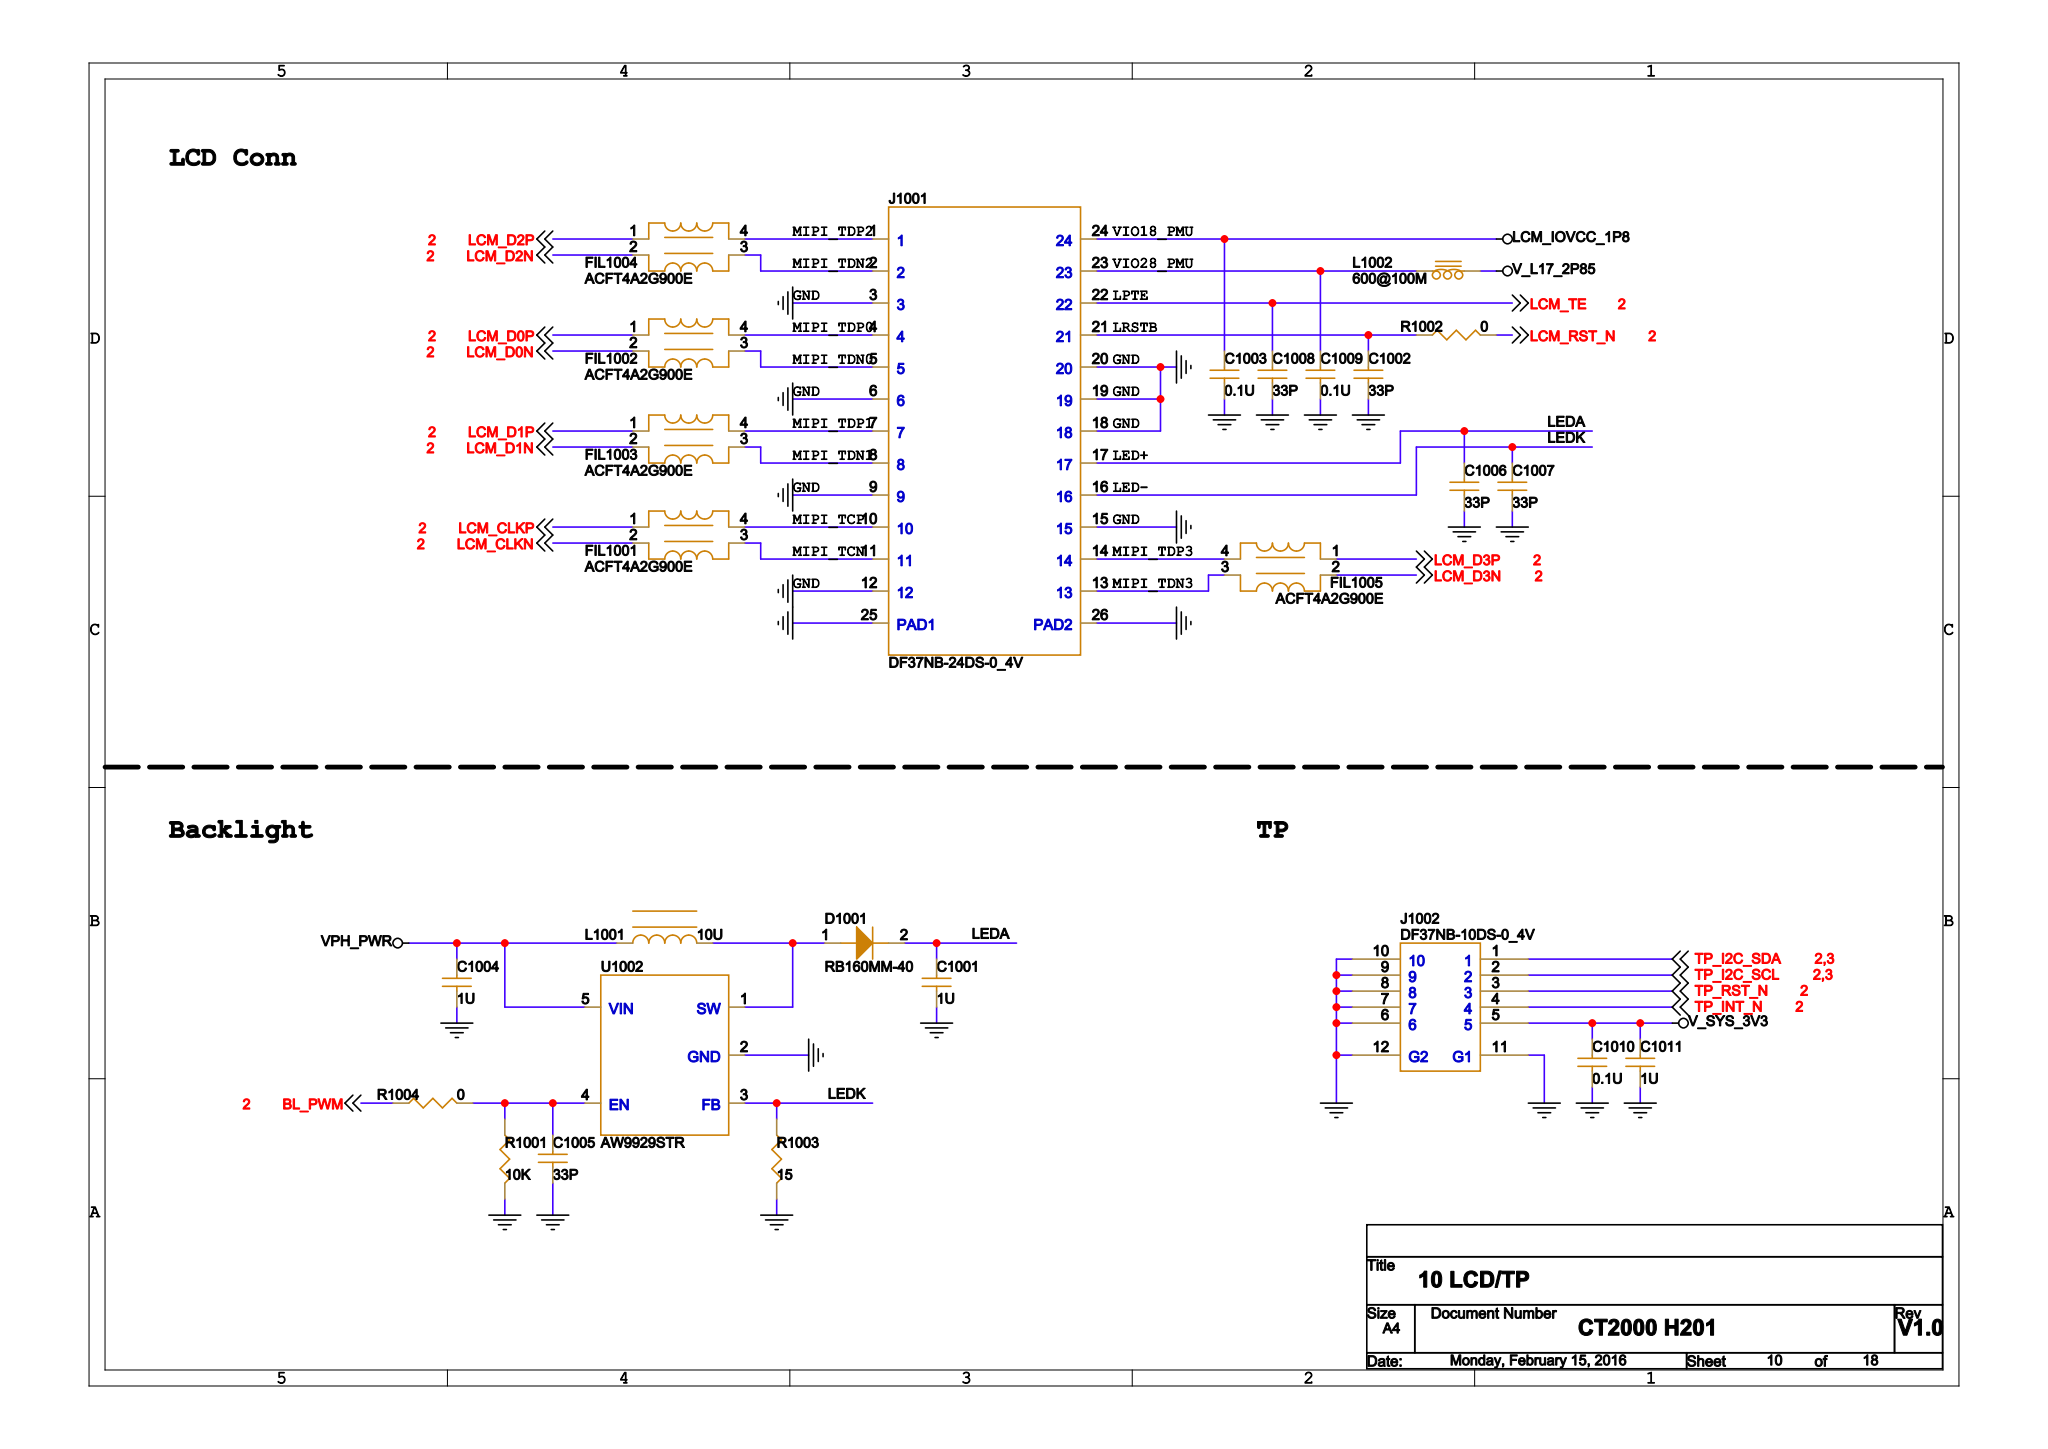Circuit board | Cadence Allegro | 573 parts | 376 nets | one sheet of the schematic
Parts on this sheet (reference | value | footprint):
C1001 | 1U | C0603
C1002 | 33P | C0402
C1003 | 0.1U | C0402
C1004 | 1U | C0402
C1005 | 33P | C0402
C1006 | 33P | C0402
C1007 | 33P | C0402
C1008 | 33P | C0402
C1009 | 0.1U | C0402
C1010 | 0.1U | C0402
C1011 | 1U | C0402
D1001 | RB160MM-40 | RB160MM-40
FIL1001 | ACFT4A2G900E | EMI4_0P85X0P65X0P55_INNOCHIPS
FIL1002 | ACFT4A2G900E | EMI4_0P85X0P65X0P55_INNOCHIPS
FIL1003 | ACFT4A2G900E | EMI4_0P85X0P65X0P55_INNOCHIPS
FIL1004 | ACFT4A2G900E | EMI4_0P85X0P65X0P55_INNOCHIPS
FIL1005 | ACFT4A2G900E | EMI4_0P85X0P65X0P55_INNOCHIPS
J1001 | DF37NB-24DS-0_4V | BTB_DF37NB-24DS-0_4V_CCW
J1002 | DF37NB-10DS-0_4V | BTB_DF37NB-10DS-0_4V_CW
L1001 | 10U | L3030_SPH3012H100MTY01
L1002 | 600@100M | L0402
R1001 | 10K | R0402
R1002 | 0 | R0402
R1003 | 15 | R0402
R1004 | 0 | R0402
U1002 | AW9929STR | SOT23_5
Nets of these parts (net: part-pin ...):
GND: C1001-2 C1002-2 C1003-2 C1004-2 C1005-2 C1006-2 C1007-2 C1008-2 C1009-2 C1010-2 C1011-2 J1002-6 J1002-7 J1002-8 J1002-9 J1002-10 J1002-11 J1002-12 R1001-2 R1003-2 U1002-2 J1001-3 J1001-6 J1001-9 J1001-12 J1001-15 J1001-18 J1001-19 J1001-20 J1001-25 J1001-26
N52618354: FIL1004-4 J1001-1
N52617518: FIL1001-4 J1001-10
N52617520: FIL1001-3 J1001-11
N52617701: FIL1005-3 J1001-13
N52617696: FIL1005-4 J1001-14
LEDK: C1007-1 R1003-1 U1002-3 J1001-16
LEDA: C1001-1 C1006-1 D1001-2 J1001-17
N52618356: FIL1004-3 J1001-2
N52617613: C1002-1 R1002-1 J1001-21
LCM_TE: C1008-1 J1001-22
N52617606: C1009-1 L1002-2 J1001-23
LCM_IOVCC_1P8: C1003-1 J1001-24
N52617432: FIL1002-4 J1001-4
N52617469: FIL1002-3 J1001-5
N52617476: FIL1003-4 J1001-7
N52617481: FIL1003-3 J1001-8
TP_I2C_SDA: J1002-1
TP_I2C_SCL: J1002-2
TP_RST_N: J1002-3
TP_INT_N: J1002-4
V_SYS_3V3: C1010-1 C1011-1 J1002-5
V_L17_2P85: L1002-1
VPH_PWR: C1004-1 L1001-1 U1002-5
BL_PWM: R1004-2
LCM_CLKN: FIL1001-2
LCM_CLKP: FIL1001-1
LCM_D0N: FIL1002-2
LCM_D0P: FIL1002-1
LCM_D1N: FIL1003-2
LCM_D1P: FIL1003-1
LCM_D2N: FIL1004-2
LCM_D2P: FIL1004-1
LCM_D3N: FIL1005-2
LCM_D3P: FIL1005-1
LCM_RST_N: R1002-2
N51987941: D1001-1 L1001-2 U1002-1
N51993764: C1005-1 R1001-1 R1004-1 U1002-4